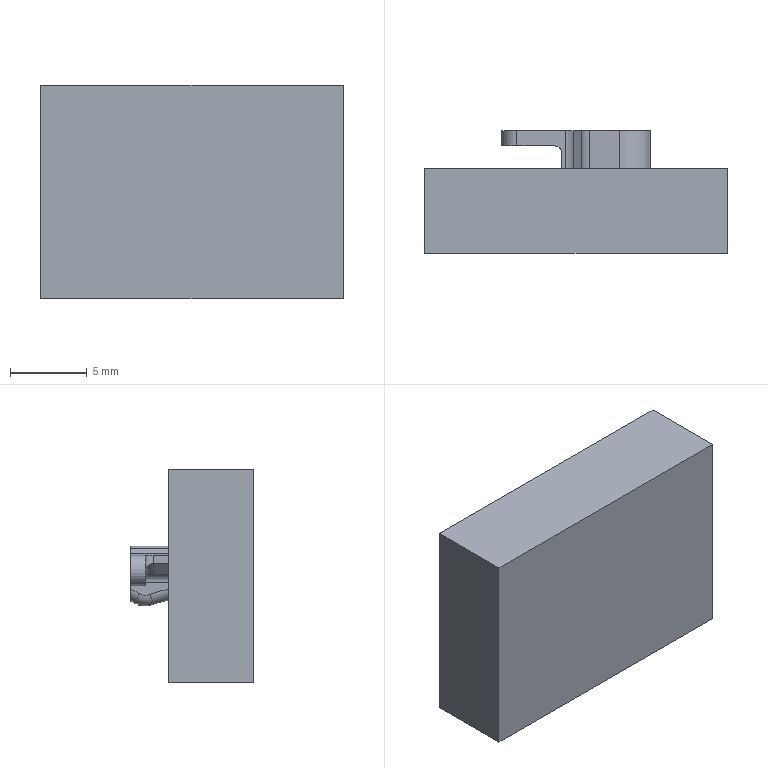NC program | NX | posted with a generic post | part box 19.7 x 8 x 13.91 mm
Whole program:
N10 G17 G21 G94 G90
(FLOOR_WALL_COPY , TOOL : D10JING)
N12 T10 M6
N14 G54
N16 G17 G0 G90 X-12.85 Y0. B0. C0. S5000 M3
N18 G43 Z30. H10
N20 Z9.781
N22 G94 G1 Z6.781 F1250.
N24 X-9.85
N26 X9.85
N28 X12.85
N30 Z9.781
N32 G0 Z30.
N34 X-12.85
N36 Z9.562
N38 G1 Z6.562
N40 X-9.85
N42 X9.85
N44 X12.85
N46 Z9.562
N48 G0 Z30.
N50 X-12.85
N52 Z9.343
N54 G1 Z6.343
N56 X-9.85
N58 X9.85
N60 X12.85
N62 Z9.343
N64 G0 Z30.
N66 X-12.85
N68 Z9.125
N70 G1 Z6.125
N72 X-9.85
N74 X9.85
N76 X12.85
N78 Z9.125
N80 G0 Z30.
N82 X-12.85
N84 Z8.906
N86 G1 Z5.906
N88 X-9.85
N90 X9.85
N92 X12.85
N94 Z8.906
N96 G0 Z30.
N98 X-12.85
N100 Z8.687
N102 G1 Z5.687
N104 X-9.85
N106 X9.85
N108 X12.85
N110 Z8.687
N112 G0 Z30.
N114 X-12.85
N116 Z8.469
N118 G1 Z5.469
N120 X-9.85
N122 X9.85
N124 X12.85
N126 Z8.469
N128 G0 Z30.
N130 X-12.85
N132 Z8.25
N134 G1 Z5.25
N136 X-9.85
N138 X9.85
N140 X12.85
N142 Z8.25
N144 G0 Z30.
N146 X-12.85
N148 Z8.031
N150 G1 Z5.031
N152 X-9.85
N154 X9.85
N156 X12.85
N158 Z8.031
N160 G0 Z30.
N162 X-12.85
N164 Z7.812
N166 G1 Z4.812
N168 X-9.85
N170 X9.85
N172 X12.85
N174 Z7.812
N176 G0 Z30.
N178 X-12.85
N180 Z7.594
N182 G1 Z4.594
N184 X-9.85
N186 X9.85
N188 X12.85
N190 Z7.594
N192 G0 Z30.
N194 X-12.85
N196 Z7.375
N198 G1 Z4.375
N200 X-9.85
N202 X9.85
N204 X12.85
N206 Z7.375
N208 G0 Z30.
N210 X-12.85
N212 Z7.156
N214 G1 Z4.156
N216 X-9.85
N218 X9.85
N220 X12.85
N222 Z7.156
N224 G0 Z30.
N226 X-12.85
N228 Z6.937
N230 G1 Z3.937
N232 X-9.85
N234 X9.85
N236 X12.85
N238 Z6.937
N240 G0 Z30.
N242 X-12.85
N244 Z6.719
N246 G1 Z3.719
N248 X-9.85
N250 X9.85
N252 X12.85
N254 Z6.719
N256 G0 Z30.
N258 X-12.85
N260 Z6.5
N262 G1 Z3.5
N264 X-9.85
N266 X9.85
N268 X12.85
N270 Z6.5
N272 G0 Z30.
N274 X-12.85
N276 Z6.281
N278 G1 Z3.281
N280 X-9.85
N282 X9.85
N284 X12.85
N286 Z6.281
N288 G0 Z30.
N290 X-12.85
N292 Z6.062
N294 G1 Z3.062
N296 X-9.85
N298 X9.85
N300 X12.85
N302 Z6.062
N304 G0 Z30.
N306 X-12.85
N308 Z5.844
N310 G1 Z2.844
N312 X-9.85
N314 X9.85
N316 X12.85
N318 Z5.844
N320 G0 Z30.
N322 X-12.85
N324 Z5.625
N326 G1 Z2.625
N328 X-9.85
N330 X9.85
N332 X12.85
N334 Z5.625
N336 G0 Z30.
N338 X-12.85
N340 Z5.406
N342 G1 Z2.406
N344 X-9.85
N346 X9.85
N348 X12.85
N350 Z5.406
N352 G0 Z30.
N354 X-12.85
N356 Z5.187
N358 G1 Z2.187
N360 X-9.85
N362 X9.85
N364 X12.85
N366 Z5.187
N368 G0 Z30.
N370 X-12.85
N372 Z4.969
N374 G1 Z1.969
N376 X-9.85
N378 X9.85
N380 X12.85
N382 Z4.969
N384 G0 Z30.
N386 X-12.85
N388 Z4.75
N390 G1 Z1.75
N392 X-9.85
N394 X9.85
N396 X12.85
N398 Z4.75
N400 G0 Z30.
N402 X-12.85
N404 Z4.531
N406 G1 Z1.531
N408 X-9.85
N410 X9.85
N412 X12.85
N414 Z4.531
N416 G0 Z30.
N418 X-12.85
N420 Z4.312
N422 G1 Z1.312
N424 X-9.85
N426 X9.85
N428 X12.85
N430 Z4.312
N432 G0 Z30.
N434 X-12.85
N436 Z4.094
N438 G1 Z1.094
N440 X-9.85
N442 X9.85
N444 X12.85
N446 Z4.094
N448 G0 Z30.
N450 X-12.85
N452 Z3.875
N454 G1 Z0.875
N456 X-9.85
N458 X9.85
N460 X12.85
N462 Z3.875
N464 G0 Z30.
N466 X-12.85
N468 Z3.656
N470 G1 Z0.656
N472 X-9.85
N474 X9.85
N476 X12.85
N478 Z3.656
N480 G0 Z30.
N482 X-12.85
N484 Z3.437
N486 G1 Z0.437
N488 X-9.85
N490 X9.85
N492 X12.85
N494 Z3.437
N496 G0 Z30.
N498 X-12.85
N500 Z3.219
N502 G1 Z0.219
N504 X-9.85
N506 X9.85
N508 X12.85
N510 Z3.219
N512 G0 Z30.
N514 X-12.85
N516 Z3.
N518 G1 Z0.
N520 X-9.85
N522 X9.85
N524 X12.85
N526 Z3.
N528 G0 Z30.
N530 M5
(PLANAR_MILL_COPY_1 , TOOL : D6A45)
N532 T07 M6
N534 G54
N536 G17 G0 G90 X1.507 Y2.612 B0. C0. S7500 M3
N538 G43 Z30. H7
N540 Z1.
N542 G94 G1 Z-1. F1250.
N544 G3 X2.273 Y2.255 R1.
N546 G1 X3.85
N548 G2 X3.358 Y-1.48 R-1.9
N550 G1 X1.322 Y-0.935
N552 G3 X0.261 Y-0.795 R4.1
N554 G1 X-2.55
N556 Y-0.85
N558 X-2.56 Y-0.981
N560 X-2.59 Y-1.189
N562 X-2.649 Y-1.438
N564 G2 X-2.812 Y-1.783 R0.9
N566 G1 X-3.023 Y-2.056
N568 G2 X-3.345 Y-2.317 R0.9
N570 G1 X-3.634 Y-2.456
N572 G2 X-4.07 Y-2.544 R0.9
N574 G1 X-4.383 Y-2.528
N576 G2 X-4.805 Y-2.398 R0.9
N578 G1 X-5.082 Y-2.23
N580 G2 X-5.373 Y-1.946 R0.9
N582 G1 X-5.562 Y-1.65
N584 G2 X-5.694 Y-1.296 R0.9
N586 G1 X-5.74 Y-0.981
N588 X-5.75 Y-0.85
N590 Y-0.045
N592 G2 X-2.85 Y2.855 R2.9
N594 G1 X-0.858
N596 G2 X0.12 Y2.584 R1.9
N598 G1 X0.645 Y2.269
N600 X0.667 Y2.249
N602 X0.696 Y2.255
N604 X2.273
N606 G3 X3.039 Y2.612 R1.
N608 G1 Z1.
N610 G0 Z30.
N612 M5
N614 M2